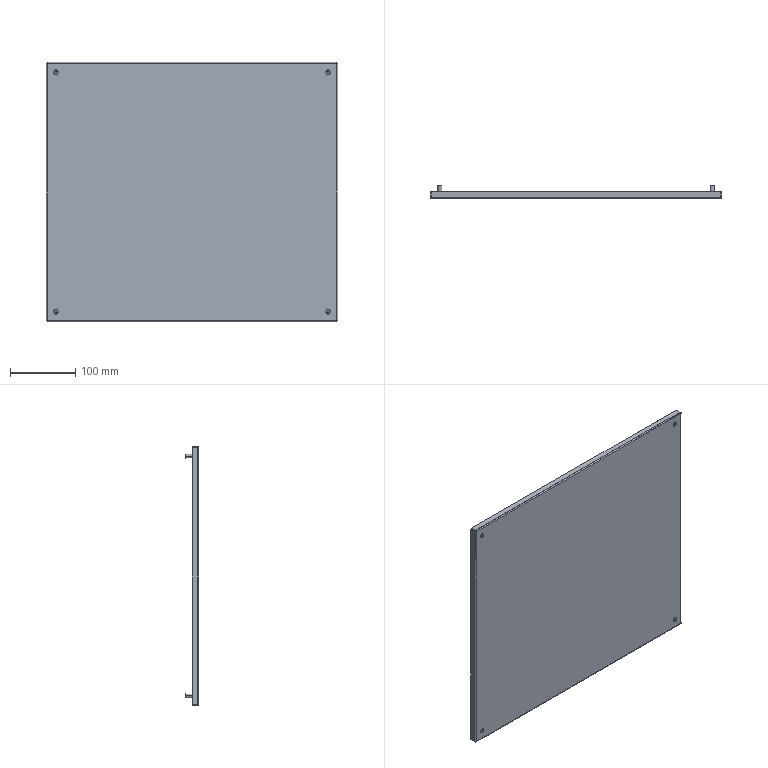Part | SolidWorks | features BaseBody 5 | 5 solids | 66 faces | box 446 x 20 x 396 mm | volume 287469 mm3 | plane 34 | cylinder 32 | commonest cylinder face diameters 1 x8 6 x8 7.2 x8 0.4 x4 3.4 x4